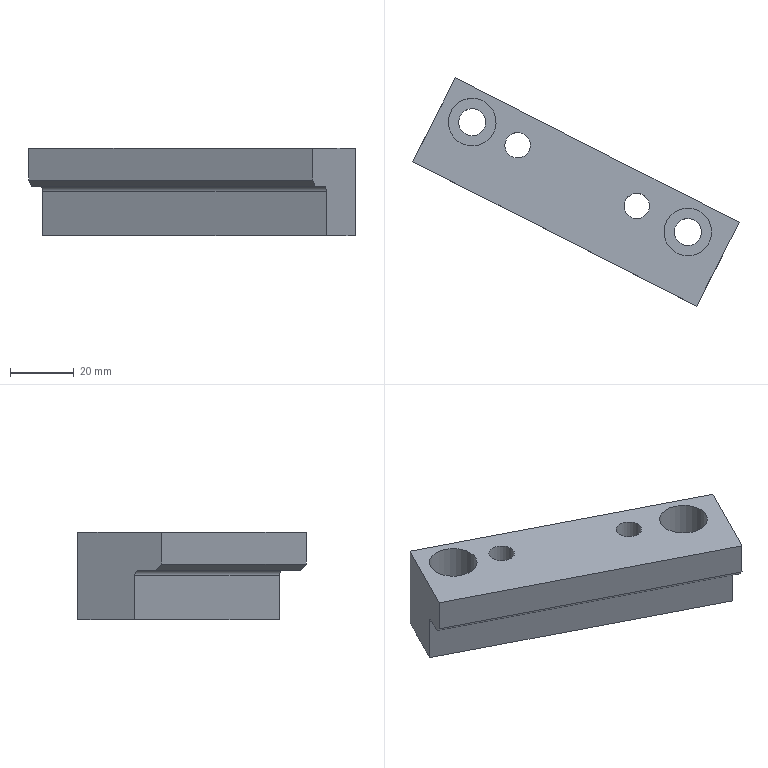Part | STEP file | gslz 2016.10.28-13_id1774_x_t | 1 solid | 18 faces | box 102.493 x 71.684 x 27.5 mm | volume 56764 mm3 | plane 11 | cylinder 7 | commonest cylinder face diameters 8 x2 8.5 x2 15 x2 3 x1
STEP:
#1=CARTESIAN_POINT('',(0.,0.,0.));
#2=DIRECTION('',(0.,0.,1.));
#3=DIRECTION('',(1.,0.,0.));
#4=AXIS2_PLACEMENT_3D('',#1,#2,#3);
#5=CARTESIAN_POINT('',(1106.799,53.815,-63.5));
#6=VERTEX_POINT('',#5);
#7=CARTESIAN_POINT('',(1105.891,52.033,-61.5));
#8=VERTEX_POINT('',#7);
#9=CARTESIAN_POINT('',(1105.891,52.033,-61.5));
#10=DIRECTION('',(-0.321,-0.63,0.7071));
#11=VECTOR('',#10,1.);
#12=LINE('',#9,#11);
#13=CARTESIAN_POINT('',(1154.896,27.063,-61.5));
#14=DIRECTION('',(-0.321,-0.63,-0.7071));
#15=DIRECTION('',(0.2523,-0.7765,0.5774));
#16=AXIS2_PLACEMENT_3D('',#13,#14,#15);
#17=PLANE('',#16);
#18=CARTESIAN_POINT('',(-31.754,44.907));
#19=DIRECTION('',(0.8165,0.5774));
#20=VECTOR('',#19,1.);
#21=LINE('',#18,#20);
#22=(GEOMETRIC_REPRESENTATION_CONTEXT(2)PARAMETRIC_REPRESENTATION_CONTEXT()REPRESENTATION_CONTEXT('',''));
#23=DEFINITIONAL_REPRESENTATION('',(#21),#22);
#24=PCURVE('',#17,#23);
#25=CARTESIAN_POINT('',(1119.283,78.318,-79.639));
#26=DIRECTION('',(0.891,-0.454,0.));
#27=DIRECTION('',(0.454,0.891,0.));
#28=AXIS2_PLACEMENT_3D('',#25,#26,#27);
#29=PLANE('',#28);
#30=CARTESIAN_POINT('',(-29.5,18.139));
#31=DIRECTION('',(-0.7071,0.7071));
#32=VECTOR('',#31,1.);
#33=LINE('',#30,#32);
#34=(GEOMETRIC_REPRESENTATION_CONTEXT(2)PARAMETRIC_REPRESENTATION_CONTEXT()REPRESENTATION_CONTEXT('',''));
#35=DEFINITIONAL_REPRESENTATION('',(#33),#34);
#36=PCURVE('',#29,#35);
#37=SURFACE_CURVE('',#12,(#24,#36),.PCURVE_S1.);
#38=EDGE_CURVE('',#6,#8,#37,.T.);
#39=ORIENTED_EDGE('',*,*,#38,.F.);
#40=CARTESIAN_POINT('',(1195.899,8.416,-63.5));
#41=VERTEX_POINT('',#40);
#42=CARTESIAN_POINT('',(1155.804,28.845,-63.5));
#43=DIRECTION('',(-0.891,0.454,0.));
#44=VECTOR('',#43,1.);
#45=LINE('',#42,#44);
#46=CARTESIAN_POINT('',(-2.309,-1.633));
#47=DIRECTION('',(-0.5774,0.8165));
#48=VECTOR('',#47,1.);
#49=LINE('',#46,#48);
#50=(GEOMETRIC_REPRESENTATION_CONTEXT(2)PARAMETRIC_REPRESENTATION_CONTEXT()REPRESENTATION_CONTEXT('',''));
#51=DEFINITIONAL_REPRESENTATION('',(#49),#50);
#52=PCURVE('',#17,#51);
#53=CARTESIAN_POINT('',(1168.289,53.348,-63.5));
#54=DIRECTION('',(0.,0.,-1.));
#55=DIRECTION('',(0.309,-0.9511,0.));
#56=AXIS2_PLACEMENT_3D('',#53,#54,#55);
#57=PLANE('',#56);
#58=CARTESIAN_POINT('',(19.445,19.445));
#59=DIRECTION('',(-0.7071,0.7071));
#60=VECTOR('',#59,1.);
#61=LINE('',#58,#60);
#62=(GEOMETRIC_REPRESENTATION_CONTEXT(2)PARAMETRIC_REPRESENTATION_CONTEXT()REPRESENTATION_CONTEXT('',''));
#63=DEFINITIONAL_REPRESENTATION('',(#61),#62);
#64=PCURVE('',#57,#63);
#65=SURFACE_CURVE('',#45,(#52,#64),.PCURVE_S1.);
#66=EDGE_CURVE('',#41,#6,#65,.T.);
#67=ORIENTED_EDGE('',*,*,#66,.F.);
#68=CARTESIAN_POINT('',(1194.991,6.634,-61.5));
#69=VERTEX_POINT('',#68);
#70=CARTESIAN_POINT('',(1205.805,27.857,-85.32));
#71=DIRECTION('',(0.321,0.63,-0.7071));
#72=VECTOR('',#71,1.);
#73=LINE('',#70,#72);
#74=CARTESIAN_POINT('',(-1.524,-56.191));
#75=DIRECTION('',(-0.8165,-0.5774));
#76=VECTOR('',#75,1.);
#77=LINE('',#74,#76);
#78=(GEOMETRIC_REPRESENTATION_CONTEXT(2)PARAMETRIC_REPRESENTATION_CONTEXT()REPRESENTATION_CONTEXT('',''));
#79=DEFINITIONAL_REPRESENTATION('',(#77),#78);
#80=PCURVE('',#17,#79);
#81=CARTESIAN_POINT('',(1208.384,32.918,-79.639));
#82=DIRECTION('',(0.891,-0.454,0.));
#83=DIRECTION('',(0.454,0.891,0.));
#84=AXIS2_PLACEMENT_3D('',#81,#82,#83);
#85=PLANE('',#84);
#86=CARTESIAN_POINT('',(-5.68,-5.68));
#87=DIRECTION('',(0.7071,-0.7071));
#88=VECTOR('',#87,1.);
#89=LINE('',#86,#88);
#90=(GEOMETRIC_REPRESENTATION_CONTEXT(2)PARAMETRIC_REPRESENTATION_CONTEXT()REPRESENTATION_CONTEXT('',''));
#91=DEFINITIONAL_REPRESENTATION('',(#89),#90);
#92=PCURVE('',#85,#91);
#93=SURFACE_CURVE('',#73,(#80,#92),.PCURVE_S1.);
#94=EDGE_CURVE('',#69,#41,#93,.T.);
#95=ORIENTED_EDGE('',*,*,#94,.F.);
#96=CARTESIAN_POINT('',(1154.896,27.063,-61.5));
#97=DIRECTION('',(0.891,-0.454,0.));
#98=VECTOR('',#97,1.);
#99=LINE('',#96,#98);
#100=CARTESIAN_POINT('',(0.,0.));
#101=DIRECTION('',(0.5774,-0.8165));
#102=VECTOR('',#101,1.);
#103=LINE('',#100,#102);
#104=(GEOMETRIC_REPRESENTATION_CONTEXT(2)PARAMETRIC_REPRESENTATION_CONTEXT()REPRESENTATION_CONTEXT('',''));
#105=DEFINITIONAL_REPRESENTATION('',(#103),#104);
#106=PCURVE('',#17,#105);
#107=CARTESIAN_POINT('',(1154.896,27.063,-51.5));
#108=DIRECTION('',(0.454,0.891,0.));
#109=DIRECTION('',(-0.891,0.454,0.));
#110=AXIS2_PLACEMENT_3D('',#107,#108,#109);
#111=PLANE('',#110);
#112=CARTESIAN_POINT('',(0.,-10.));
#113=DIRECTION('',(-1.,0.));
#114=VECTOR('',#113,1.);
#115=LINE('',#112,#114);
#116=(GEOMETRIC_REPRESENTATION_CONTEXT(2)PARAMETRIC_REPRESENTATION_CONTEXT()REPRESENTATION_CONTEXT('',''));
#117=DEFINITIONAL_REPRESENTATION('',(#115),#116);
#118=PCURVE('',#111,#117);
#119=SURFACE_CURVE('',#99,(#106,#118),.PCURVE_S1.);
#120=EDGE_CURVE('',#8,#69,#119,.T.);
#121=ORIENTED_EDGE('',*,*,#120,.F.);
#122=EDGE_LOOP('',(#39,#67,#95,#121));
#123=FACE_BOUND('',#122,.T.);
#124=ADVANCED_FACE('',(#123),#17,.T.);
#125=CARTESIAN_POINT('',(1198.623,13.762,-63.5));
#126=VERTEX_POINT('',#125);
#127=CARTESIAN_POINT('',(1208.384,32.918,-63.5));
#128=DIRECTION('',(-0.454,-0.891,0.));
#129=VECTOR('',#128,1.);
#130=LINE('',#127,#129);
#131=CARTESIAN_POINT('',(31.82,-31.82));
#132=DIRECTION('',(0.7071,0.7071));
#133=VECTOR('',#132,1.);
#134=LINE('',#131,#133);
#135=(GEOMETRIC_REPRESENTATION_CONTEXT(2)PARAMETRIC_REPRESENTATION_CONTEXT()REPRESENTATION_CONTEXT('',''));
#136=DEFINITIONAL_REPRESENTATION('',(#134),#135);
#137=PCURVE('',#57,#136);
#138=CARTESIAN_POINT('',(0.,16.139));
#139=DIRECTION('',(-1.,0.));
#140=VECTOR('',#139,1.);
#141=LINE('',#138,#140);
#142=(GEOMETRIC_REPRESENTATION_CONTEXT(2)PARAMETRIC_REPRESENTATION_CONTEXT()REPRESENTATION_CONTEXT('',''));
#143=DEFINITIONAL_REPRESENTATION('',(#141),#142);
#144=PCURVE('',#85,#143);
#145=SURFACE_CURVE('',#130,(#137,#144),.PCURVE_S1.);
#146=EDGE_CURVE('',#126,#41,#145,.T.);
#147=ORIENTED_EDGE('',*,*,#146,.T.);
#148=ORIENTED_EDGE('',*,*,#66,.T.);
#149=CARTESIAN_POINT('',(1109.523,59.161,-63.5));
#150=VERTEX_POINT('',#149);
#151=CARTESIAN_POINT('',(1119.283,78.318,-63.5));
#152=DIRECTION('',(-0.454,-0.891,0.));
#153=VECTOR('',#152,1.);
#154=LINE('',#151,#153);
#155=CARTESIAN_POINT('',(-38.891,38.891));
#156=DIRECTION('',(0.7071,0.7071));
#157=VECTOR('',#156,1.);
#158=LINE('',#155,#157);
#159=(GEOMETRIC_REPRESENTATION_CONTEXT(2)PARAMETRIC_REPRESENTATION_CONTEXT()REPRESENTATION_CONTEXT('',''));
#160=DEFINITIONAL_REPRESENTATION('',(#158),#159);
#161=PCURVE('',#57,#160);
#162=CARTESIAN_POINT('',(0.,16.139));
#163=DIRECTION('',(-1.,0.));
#164=VECTOR('',#163,1.);
#165=LINE('',#162,#164);
#166=(GEOMETRIC_REPRESENTATION_CONTEXT(2)PARAMETRIC_REPRESENTATION_CONTEXT()REPRESENTATION_CONTEXT('',''));
#167=DEFINITIONAL_REPRESENTATION('',(#165),#166);
#168=PCURVE('',#29,#167);
#169=SURFACE_CURVE('',#154,(#161,#168),.PCURVE_S1.);
#170=EDGE_CURVE('',#150,#6,#169,.T.);
#171=ORIENTED_EDGE('',*,*,#170,.F.);
#172=CARTESIAN_POINT('',(1158.528,34.191,-63.5));
#173=DIRECTION('',(0.891,-0.454,0.));
#174=VECTOR('',#173,1.);
#175=LINE('',#172,#174);
#176=CARTESIAN_POINT('',(15.203,15.203));
#177=DIRECTION('',(0.7071,-0.7071));
#178=VECTOR('',#177,1.);
#179=LINE('',#176,#178);
#180=(GEOMETRIC_REPRESENTATION_CONTEXT(2)PARAMETRIC_REPRESENTATION_CONTEXT()REPRESENTATION_CONTEXT('',''));
#181=DEFINITIONAL_REPRESENTATION('',(#179),#180);
#182=PCURVE('',#57,#181);
#183=CARTESIAN_POINT('',(1158.528,34.191,-65.));
#184=DIRECTION('',(0.891,-0.454,0.));
#185=DIRECTION('',(0.454,0.891,0.));
#186=AXIS2_PLACEMENT_3D('',#183,#184,#185);
#187=CYLINDRICAL_SURFACE('',#186,1.5);
#188=CARTESIAN_POINT('',(1.571,0.));
#189=DIRECTION('',(0.,1.));
#190=VECTOR('',#189,1.);
#191=LINE('',#188,#190);
#192=(GEOMETRIC_REPRESENTATION_CONTEXT(2)PARAMETRIC_REPRESENTATION_CONTEXT()REPRESENTATION_CONTEXT('',''));
#193=DEFINITIONAL_REPRESENTATION('',(#191),#192);
#194=PCURVE('',#187,#193);
#195=SURFACE_CURVE('',#175,(#182,#194),.PCURVE_S1.);
#196=EDGE_CURVE('',#150,#126,#195,.T.);
#197=ORIENTED_EDGE('',*,*,#196,.T.);
#198=EDGE_LOOP('',(#147,#148,#171,#197));
#199=FACE_BOUND('',#198,.T.);
#200=ADVANCED_FACE('',(#199),#57,.T.);
#201=ORIENTED_EDGE('',*,*,#196,.T.);
#202=CARTESIAN_POINT('',(1199.304,15.098,-65.));
#203=VERTEX_POINT('',#202);
#204=CARTESIAN_POINT('',(1198.623,13.762,-65.));
#205=DIRECTION('',(-0.891,0.454,0.));
#206=DIRECTION('',(0.454,0.891,0.));
#207=AXIS2_PLACEMENT_3D('',#204,#205,#206);
#208=CIRCLE('',#207,1.5);
#209=CARTESIAN_POINT('',(6.283,45.));
#210=DIRECTION('',(-1.,0.));
#211=VECTOR('',#210,1.);
#212=LINE('',#209,#211);
#213=(GEOMETRIC_REPRESENTATION_CONTEXT(2)PARAMETRIC_REPRESENTATION_CONTEXT()REPRESENTATION_CONTEXT('',''));
#214=DEFINITIONAL_REPRESENTATION('',(#212),#213);
#215=PCURVE('',#187,#214);
#216=CARTESIAN_POINT('',(-20.,14.639));
#217=CARTESIAN_POINT('',(-20.,12.041));
#218=CARTESIAN_POINT('',(-22.25,13.34));
#219=CARTESIAN_POINT('',(-24.5,14.639));
#220=CARTESIAN_POINT('',(-22.25,15.938));
#221=CARTESIAN_POINT('',(-20.,17.237));
#222=CARTESIAN_POINT('',(-20.,14.639));
#223=(BOUNDED_CURVE()B_SPLINE_CURVE(2,(#216,#217,#218,#219,#220,#221,#222),.UNSPECIFIED.,.T.,.F.)B_SPLINE_CURVE_WITH_KNOTS((1,2,2,2,2,1),(-2.094,0.,2.094,4.189,6.283,8.378),.UNSPECIFIED.)CURVE()GEOMETRIC_REPRESENTATION_ITEM()RATIONAL_B_SPLINE_CURVE((1.,0.5,1.,0.5,1.,0.5,1.))REPRESENTATION_ITEM(''));
#224=(GEOMETRIC_REPRESENTATION_CONTEXT(2)PARAMETRIC_REPRESENTATION_CONTEXT()REPRESENTATION_CONTEXT('',''));
#225=DEFINITIONAL_REPRESENTATION('',(#223),#224);
#226=PCURVE('',#85,#225);
#227=SURFACE_CURVE('',#208,(#215,#226),.PCURVE_S1.);
#228=EDGE_CURVE('',#126,#203,#227,.T.);
#229=ORIENTED_EDGE('',*,*,#228,.T.);
#230=CARTESIAN_POINT('',(1110.204,60.497,-65.));
#231=VERTEX_POINT('',#230);
#232=CARTESIAN_POINT('',(1159.209,35.528,-65.));
#233=DIRECTION('',(-0.891,0.454,0.));
#234=VECTOR('',#233,1.);
#235=LINE('',#232,#234);
#236=CARTESIAN_POINT('',(0.,0.));
#237=DIRECTION('',(0.,-1.));
#238=VECTOR('',#237,1.);
#239=LINE('',#236,#238);
#240=(GEOMETRIC_REPRESENTATION_CONTEXT(2)PARAMETRIC_REPRESENTATION_CONTEXT()REPRESENTATION_CONTEXT('',''));
#241=DEFINITIONAL_REPRESENTATION('',(#239),#240);
#242=PCURVE('',#187,#241);
#243=CARTESIAN_POINT('',(1159.209,35.528,-79.639));
#244=DIRECTION('',(0.454,0.891,0.));
#245=DIRECTION('',(-0.891,0.454,0.));
#246=AXIS2_PLACEMENT_3D('',#243,#244,#245);
#247=PLANE('',#246);
#248=CARTESIAN_POINT('',(0.,14.639));
#249=DIRECTION('',(1.,0.));
#250=VECTOR('',#249,1.);
#251=LINE('',#248,#250);
#252=(GEOMETRIC_REPRESENTATION_CONTEXT(2)PARAMETRIC_REPRESENTATION_CONTEXT()REPRESENTATION_CONTEXT('',''));
#253=DEFINITIONAL_REPRESENTATION('',(#251),#252);
#254=PCURVE('',#247,#253);
#255=SURFACE_CURVE('',#235,(#242,#254),.PCURVE_S1.);
#256=EDGE_CURVE('',#203,#231,#255,.T.);
#257=ORIENTED_EDGE('',*,*,#256,.T.);
#258=CARTESIAN_POINT('',(1109.523,59.161,-65.));
#259=DIRECTION('',(0.891,-0.454,0.));
#260=DIRECTION('',(0.454,0.891,0.));
#261=AXIS2_PLACEMENT_3D('',#258,#259,#260);
#262=CIRCLE('',#261,1.5);
#263=CARTESIAN_POINT('',(0.,-55.));
#264=DIRECTION('',(1.,0.));
#265=VECTOR('',#264,1.);
#266=LINE('',#263,#265);
#267=(GEOMETRIC_REPRESENTATION_CONTEXT(2)PARAMETRIC_REPRESENTATION_CONTEXT()REPRESENTATION_CONTEXT('',''));
#268=DEFINITIONAL_REPRESENTATION('',(#266),#267);
#269=PCURVE('',#187,#268);
#270=CARTESIAN_POINT('',(-21.5,14.639));
#271=DIRECTION('',(1.,0.));
#272=AXIS2_PLACEMENT_2D('',#270,#271);
#273=CIRCLE('',#272,1.5);
#274=(GEOMETRIC_REPRESENTATION_CONTEXT(2)PARAMETRIC_REPRESENTATION_CONTEXT()REPRESENTATION_CONTEXT('',''));
#275=DEFINITIONAL_REPRESENTATION('',(#273),#274);
#276=PCURVE('',#29,#275);
#277=SURFACE_CURVE('',#262,(#269,#276),.PCURVE_S1.);
#278=EDGE_CURVE('',#231,#150,#277,.T.);
#279=ORIENTED_EDGE('',*,*,#278,.T.);
#280=EDGE_LOOP('',(#201,#229,#257,#279));
#281=FACE_BOUND('',#280,.F.);
#282=ADVANCED_FACE('',(#281),#187,.F.);
#283=CARTESIAN_POINT('',(1193.574,25.868,-66.5));
#284=VERTEX_POINT('',#283);
#285=CARTESIAN_POINT('',(1192.261,29.91,-66.5));
#286=DIRECTION('',(0.,0.,1.));
#287=DIRECTION('',(0.309,-0.9511,0.));
#288=AXIS2_PLACEMENT_3D('',#285,#286,#287);
#289=CIRCLE('',#288,4.25);
#290=CARTESIAN_POINT('',(1192.261,29.91,-66.5));
#291=DIRECTION('',(0.,0.,-1.));
#292=DIRECTION('',(0.309,-0.9511,0.));
#293=AXIS2_PLACEMENT_3D('',#290,#291,#292);
#294=PLANE('',#293);
#295=CARTESIAN_POINT('',(4.25,0.));
#296=CARTESIAN_POINT('',(4.25,-7.361));
#297=CARTESIAN_POINT('',(-2.125,-3.681));
#298=CARTESIAN_POINT('',(-8.5,0.));
#299=CARTESIAN_POINT('',(-2.125,3.681));
#300=CARTESIAN_POINT('',(4.25,7.361));
#301=CARTESIAN_POINT('',(4.25,0.));
#302=(BOUNDED_CURVE()B_SPLINE_CURVE(2,(#295,#296,#297,#298,#299,#300,#301),.UNSPECIFIED.,.T.,.F.)B_SPLINE_CURVE_WITH_KNOTS((1,2,2,2,2,1),(-2.094,0.,2.094,4.189,6.283,8.378),.UNSPECIFIED.)CURVE()GEOMETRIC_REPRESENTATION_ITEM()RATIONAL_B_SPLINE_CURVE((1.,0.5,1.,0.5,1.,0.5,1.))REPRESENTATION_ITEM(''));
#303=(GEOMETRIC_REPRESENTATION_CONTEXT(2)PARAMETRIC_REPRESENTATION_CONTEXT()REPRESENTATION_CONTEXT('',''));
#304=DEFINITIONAL_REPRESENTATION('',(#302),#303);
#305=PCURVE('',#294,#304);
#306=CARTESIAN_POINT('',(1192.261,29.91,-101.5));
#307=DIRECTION('',(0.,0.,-1.));
#308=DIRECTION('',(0.309,-0.9511,0.));
#309=AXIS2_PLACEMENT_3D('',#306,#307,#308);
#310=CYLINDRICAL_SURFACE('',#309,4.25);
#311=CARTESIAN_POINT('',(6.283,-35.));
#312=DIRECTION('',(-1.,0.));
#313=VECTOR('',#312,1.);
#314=LINE('',#311,#313);
#315=(GEOMETRIC_REPRESENTATION_CONTEXT(2)PARAMETRIC_REPRESENTATION_CONTEXT()REPRESENTATION_CONTEXT('',''));
#316=DEFINITIONAL_REPRESENTATION('',(#314),#315);
#317=PCURVE('',#310,#316);
#318=SURFACE_CURVE('',#289,(#305,#317),.PCURVE_S1.);
#319=EDGE_CURVE('',#284,#284,#318,.T.);
#320=ORIENTED_EDGE('',*,*,#319,.F.);
#321=EDGE_LOOP('',(#320));
#322=FACE_BOUND('',#321,.T.);
#323=CARTESIAN_POINT('',(1194.579,22.777,-66.5));
#324=VERTEX_POINT('',#323);
#325=CARTESIAN_POINT('',(1192.261,29.91,-66.5));
#326=DIRECTION('',(0.,0.,1.));
#327=DIRECTION('',(0.309,-0.9511,0.));
#328=AXIS2_PLACEMENT_3D('',#325,#326,#327);
#329=CIRCLE('',#328,7.5);
#330=CARTESIAN_POINT('',(7.5,0.));
#331=CARTESIAN_POINT('',(7.5,-12.99));
#332=CARTESIAN_POINT('',(-3.75,-6.495));
#333=CARTESIAN_POINT('',(-15.,0.));
#334=CARTESIAN_POINT('',(-3.75,6.495));
#335=CARTESIAN_POINT('',(7.5,12.99));
#336=CARTESIAN_POINT('',(7.5,0.));
#337=(BOUNDED_CURVE()B_SPLINE_CURVE(2,(#330,#331,#332,#333,#334,#335,#336),.UNSPECIFIED.,.T.,.F.)B_SPLINE_CURVE_WITH_KNOTS((1,2,2,2,2,1),(-2.094,0.,2.094,4.189,6.283,8.378),.UNSPECIFIED.)CURVE()GEOMETRIC_REPRESENTATION_ITEM()RATIONAL_B_SPLINE_CURVE((1.,0.5,1.,0.5,1.,0.5,1.))REPRESENTATION_ITEM(''));
#338=(GEOMETRIC_REPRESENTATION_CONTEXT(2)PARAMETRIC_REPRESENTATION_CONTEXT()REPRESENTATION_CONTEXT('',''));
#339=DEFINITIONAL_REPRESENTATION('',(#337),#338);
#340=PCURVE('',#294,#339);
#341=CARTESIAN_POINT('',(1192.261,29.91,-51.5));
#342=DIRECTION('',(0.,0.,-1.));
#343=DIRECTION('',(0.309,-0.9511,0.));
#344=AXIS2_PLACEMENT_3D('',#341,#342,#343);
#345=CYLINDRICAL_SURFACE('',#344,7.5);
#346=CARTESIAN_POINT('',(6.283,15.));
#347=DIRECTION('',(-1.,0.));
#348=VECTOR('',#347,1.);
#349=LINE('',#346,#348);
#350=(GEOMETRIC_REPRESENTATION_CONTEXT(2)PARAMETRIC_REPRESENTATION_CONTEXT()REPRESENTATION_CONTEXT('',''));
#351=DEFINITIONAL_REPRESENTATION('',(#349),#350);
#352=PCURVE('',#345,#351);
#353=SURFACE_CURVE('',#329,(#340,#352),.PCURVE_S1.);
#354=EDGE_CURVE('',#324,#324,#353,.T.);
#355=ORIENTED_EDGE('',*,*,#354,.T.);
#356=EDGE_LOOP('',(#355));
#357=FACE_BOUND('',#356,.T.);
#358=ADVANCED_FACE('',(#322,#357),#294,.F.);
#359=CARTESIAN_POINT('',(1125.858,60.372,-66.5));
#360=VERTEX_POINT('',#359);
#361=CARTESIAN_POINT('',(1124.545,64.414,-66.5));
#362=DIRECTION('',(0.,0.,1.));
#363=DIRECTION('',(0.309,-0.9511,0.));
#364=AXIS2_PLACEMENT_3D('',#361,#362,#363);
#365=CIRCLE('',#364,4.25);
#366=CARTESIAN_POINT('',(1142.365,55.334,-66.5));
#367=DIRECTION('',(0.,0.,-1.));
#368=DIRECTION('',(0.309,-0.9511,0.));
#369=AXIS2_PLACEMENT_3D('',#366,#367,#368);
#370=PLANE('',#369);
#371=CARTESIAN_POINT('',(-9.892,14.142));
#372=CARTESIAN_POINT('',(-9.892,6.781));
#373=CARTESIAN_POINT('',(-16.267,10.462));
#374=CARTESIAN_POINT('',(-22.642,14.142));
#375=CARTESIAN_POINT('',(-16.267,17.823));
#376=CARTESIAN_POINT('',(-9.892,21.503));
#377=CARTESIAN_POINT('',(-9.892,14.142));
#378=(BOUNDED_CURVE()B_SPLINE_CURVE(2,(#371,#372,#373,#374,#375,#376,#377),.UNSPECIFIED.,.T.,.F.)B_SPLINE_CURVE_WITH_KNOTS((1,2,2,2,2,1),(-2.094,0.,2.094,4.189,6.283,8.378),.UNSPECIFIED.)CURVE()GEOMETRIC_REPRESENTATION_ITEM()RATIONAL_B_SPLINE_CURVE((1.,0.5,1.,0.5,1.,0.5,1.))REPRESENTATION_ITEM(''));
#379=(GEOMETRIC_REPRESENTATION_CONTEXT(2)PARAMETRIC_REPRESENTATION_CONTEXT()REPRESENTATION_CONTEXT('',''));
#380=DEFINITIONAL_REPRESENTATION('',(#378),#379);
#381=PCURVE('',#370,#380);
#382=CARTESIAN_POINT('',(1124.545,64.414,-101.5));
#383=DIRECTION('',(0.,0.,-1.));
#384=DIRECTION('',(0.309,-0.9511,0.));
#385=AXIS2_PLACEMENT_3D('',#382,#383,#384);
#386=CYLINDRICAL_SURFACE('',#385,4.25);
#387=CARTESIAN_POINT('',(6.283,-35.));
#388=DIRECTION('',(-1.,0.));
#389=VECTOR('',#388,1.);
#390=LINE('',#387,#389);
#391=(GEOMETRIC_REPRESENTATION_CONTEXT(2)PARAMETRIC_REPRESENTATION_CONTEXT()REPRESENTATION_CONTEXT('',''));
#392=DEFINITIONAL_REPRESENTATION('',(#390),#391);
#393=PCURVE('',#386,#392);
#394=SURFACE_CURVE('',#365,(#381,#393),.PCURVE_S1.);
#395=EDGE_CURVE('',#360,#360,#394,.T.);
#396=ORIENTED_EDGE('',*,*,#395,.F.);
#397=EDGE_LOOP('',(#396));
#398=FACE_BOUND('',#397,.T.);
#399=CARTESIAN_POINT('',(1126.862,57.281,-66.5));
#400=VERTEX_POINT('',#399);
#401=CARTESIAN_POINT('',(1124.545,64.414,-66.5));
#402=DIRECTION('',(0.,0.,1.));
#403=DIRECTION('',(0.309,-0.9511,0.));
#404=AXIS2_PLACEMENT_3D('',#401,#402,#403);
#405=CIRCLE('',#404,7.5);
#406=CARTESIAN_POINT('',(-6.642,14.142));
#407=CARTESIAN_POINT('',(-6.642,1.152));
#408=CARTESIAN_POINT('',(-17.892,7.647));
#409=CARTESIAN_POINT('',(-29.142,14.142));
#410=CARTESIAN_POINT('',(-17.892,20.637));
#411=CARTESIAN_POINT('',(-6.642,27.133));
#412=CARTESIAN_POINT('',(-6.642,14.142));
#413=(BOUNDED_CURVE()B_SPLINE_CURVE(2,(#406,#407,#408,#409,#410,#411,#412),.UNSPECIFIED.,.T.,.F.)B_SPLINE_CURVE_WITH_KNOTS((1,2,2,2,2,1),(-2.094,0.,2.094,4.189,6.283,8.378),.UNSPECIFIED.)CURVE()GEOMETRIC_REPRESENTATION_ITEM()RATIONAL_B_SPLINE_CURVE((1.,0.5,1.,0.5,1.,0.5,1.))REPRESENTATION_ITEM(''));
#414=(GEOMETRIC_REPRESENTATION_CONTEXT(2)PARAMETRIC_REPRESENTATION_CONTEXT()REPRESENTATION_CONTEXT('',''));
#415=DEFINITIONAL_REPRESENTATION('',(#413),#414);
#416=PCURVE('',#370,#415);
#417=CARTESIAN_POINT('',(1124.545,64.414,-51.5));
#418=DIRECTION('',(0.,0.,-1.));
#419=DIRECTION('',(0.309,-0.9511,0.));
#420=AXIS2_PLACEMENT_3D('',#417,#418,#419);
#421=CYLINDRICAL_SURFACE('',#420,7.5);
#422=CARTESIAN_POINT('',(6.283,15.));
#423=DIRECTION('',(-1.,0.));
#424=VECTOR('',#423,1.);
#425=LINE('',#422,#424);
#426=(GEOMETRIC_REPRESENTATION_CONTEXT(2)PARAMETRIC_REPRESENTATION_CONTEXT()REPRESENTATION_CONTEXT('',''));
#427=DEFINITIONAL_REPRESENTATION('',(#425),#426);
#428=PCURVE('',#421,#427);
#429=SURFACE_CURVE('',#405,(#416,#428),.PCURVE_S1.);
#430=EDGE_CURVE('',#400,#400,#429,.T.);
#431=ORIENTED_EDGE('',*,*,#430,.T.);
#432=EDGE_LOOP('',(#431));
#433=FACE_BOUND('',#432,.T.);
#434=ADVANCED_FACE('',(#398,#433),#370,.F.);
#435=CARTESIAN_POINT('',(1194.991,6.634,-51.5));
#436=VERTEX_POINT('',#435);
#437=CARTESIAN_POINT('',(1194.991,6.634,-51.5));
#438=DIRECTION('',(0.,0.,-1.));
#439=VECTOR('',#438,1.);
#440=LINE('',#437,#439);
#441=CARTESIAN_POINT('',(-45.,0.));
#442=DIRECTION('',(0.,-1.));
#443=VECTOR('',#442,1.);
#444=LINE('',#441,#443);
#445=(GEOMETRIC_REPRESENTATION_CONTEXT(2)PARAMETRIC_REPRESENTATION_CONTEXT()REPRESENTATION_CONTEXT('',''));
#446=DEFINITIONAL_REPRESENTATION('',(#444),#445);
#447=PCURVE('',#111,#446);
#448=CARTESIAN_POINT('',(-29.5,28.139));
#449=DIRECTION('',(0.,-1.));
#450=VECTOR('',#449,1.);
#451=LINE('',#448,#450);
#452=(GEOMETRIC_REPRESENTATION_CONTEXT(2)PARAMETRIC_REPRESENTATION_CONTEXT()REPRESENTATION_CONTEXT('',''));
#453=DEFINITIONAL_REPRESENTATION('',(#451),#452);
#454=PCURVE('',#85,#453);
#455=SURFACE_CURVE('',#440,(#447,#454),.PCURVE_S1.);
#456=EDGE_CURVE('',#436,#69,#455,.T.);
#457=ORIENTED_EDGE('',*,*,#456,.F.);
#458=CARTESIAN_POINT('',(1105.891,52.033,-51.5));
#459=VERTEX_POINT('',#458);
#460=CARTESIAN_POINT('',(1154.896,27.063,-51.5));
#461=DIRECTION('',(-0.891,0.454,0.));
#462=VECTOR('',#461,1.);
#463=LINE('',#460,#462);
#464=CARTESIAN_POINT('',(0.,0.));
#465=DIRECTION('',(1.,0.));
#466=VECTOR('',#465,1.);
#467=LINE('',#464,#466);
#468=(GEOMETRIC_REPRESENTATION_CONTEXT(2)PARAMETRIC_REPRESENTATION_CONTEXT()REPRESENTATION_CONTEXT('',''));
#469=DEFINITIONAL_REPRESENTATION('',(#467),#468);
#470=PCURVE('',#111,#469);
#471=CARTESIAN_POINT('',(1168.289,53.348,-51.5));
#472=DIRECTION('',(0.,0.,-1.));
#473=DIRECTION('',(0.309,-0.9511,0.));
#474=AXIS2_PLACEMENT_3D('',#471,#472,#473);
#475=PLANE('',#474);
#476=CARTESIAN_POINT('',(20.86,20.86));
#477=DIRECTION('',(-0.7071,0.7071));
#478=VECTOR('',#477,1.);
#479=LINE('',#476,#478);
#480=(GEOMETRIC_REPRESENTATION_CONTEXT(2)PARAMETRIC_REPRESENTATION_CONTEXT()REPRESENTATION_CONTEXT('',''));
#481=DEFINITIONAL_REPRESENTATION('',(#479),#480);
#482=PCURVE('',#475,#481);
#483=SURFACE_CURVE('',#463,(#470,#482),.PCURVE_S1.);
#484=EDGE_CURVE('',#436,#459,#483,.T.);
#485=ORIENTED_EDGE('',*,*,#484,.T.);
#486=CARTESIAN_POINT('',(1105.891,52.033,-51.5));
#487=DIRECTION('',(0.,0.,-1.));
#488=VECTOR('',#487,1.);
#489=LINE('',#486,#488);
#490=CARTESIAN_POINT('',(55.,0.));
#491=DIRECTION('',(0.,-1.));
#492=VECTOR('',#491,1.);
#493=LINE('',#490,#492);
#494=(GEOMETRIC_REPRESENTATION_CONTEXT(2)PARAMETRIC_REPRESENTATION_CONTEXT()REPRESENTATION_CONTEXT('',''));
#495=DEFINITIONAL_REPRESENTATION('',(#493),#494);
#496=PCURVE('',#111,#495);
#497=CARTESIAN_POINT('',(-29.5,28.139));
#498=DIRECTION('',(0.,-1.));
#499=VECTOR('',#498,1.);
#500=LINE('',#497,#499);
#501=(GEOMETRIC_REPRESENTATION_CONTEXT(2)PARAMETRIC_REPRESENTATION_CONTEXT()REPRESENTATION_CONTEXT('',''));
#502=DEFINITIONAL_REPRESENTATION('',(#500),#501);
#503=PCURVE('',#29,#502);
#504=SURFACE_CURVE('',#489,(#496,#503),.PCURVE_S1.);
#505=EDGE_CURVE('',#459,#8,#504,.T.);
#506=ORIENTED_EDGE('',*,*,#505,.T.);
#507=ORIENTED_EDGE('',*,*,#120,.T.);
#508=EDGE_LOOP('',(#457,#485,#506,#507));
#509=FACE_BOUND('',#508,.T.);
#510=ADVANCED_FACE('',(#509),#111,.F.);
#511=ORIENTED_EDGE('',*,*,#354,.T.);
#512=CARTESIAN_POINT('',(1194.579,22.777,-51.5));
#513=VERTEX_POINT('',#512);
#514=CARTESIAN_POINT('',(1194.579,22.777,-51.5));
#515=CARTESIAN_POINT('',(1194.579,22.777,-66.5));
#516=B_SPLINE_CURVE_WITH_KNOTS('',1,(#514,#515),.UNSPECIFIED.,.F.,.F.,(2,2),(0.,15.),.PIECEWISE_BEZIER_KNOTS.);
#517=CARTESIAN_POINT('',(0.,0.));
#518=DIRECTION('',(0.,1.));
#519=VECTOR('',#518,1.);
#520=LINE('',#517,#519);
#521=(GEOMETRIC_REPRESENTATION_CONTEXT(2)PARAMETRIC_REPRESENTATION_CONTEXT()REPRESENTATION_CONTEXT('',''));
#522=DEFINITIONAL_REPRESENTATION('',(#520),#521);
#523=PCURVE('',#345,#522);
#524=CARTESIAN_POINT('',(6.283,0.));
#525=DIRECTION('',(0.,1.));
#526=VECTOR('',#525,1.);
#527=LINE('',#524,#526);
#528=(GEOMETRIC_REPRESENTATION_CONTEXT(2)PARAMETRIC_REPRESENTATION_CONTEXT()REPRESENTATION_CONTEXT('',''));
#529=DEFINITIONAL_REPRESENTATION('',(#527),#528);
#530=PCURVE('',#345,#529);
#531=SEAM_CURVE('',#516,(#523,#530),.PCURVE_S1.);
#532=EDGE_CURVE('',#513,#324,#531,.T.);
#533=ORIENTED_EDGE('',*,*,#532,.F.);
#534=CARTESIAN_POINT('',(1192.261,29.91,-51.5));
#535=DIRECTION('',(0.,0.,-1.));
#536=DIRECTION('',(0.309,-0.9511,0.));
#537=AXIS2_PLACEMENT_3D('',#534,#535,#536);
#538=CIRCLE('',#537,7.5);
#539=CARTESIAN_POINT('',(0.,0.));
#540=DIRECTION('',(1.,0.));
#541=VECTOR('',#540,1.);
#542=LINE('',#539,#541);
#543=(GEOMETRIC_REPRESENTATION_CONTEXT(2)PARAMETRIC_REPRESENTATION_CONTEXT()REPRESENTATION_CONTEXT('',''));
#544=DEFINITIONAL_REPRESENTATION('',(#542),#543);
#545=PCURVE('',#345,#544);
#546=CARTESIAN_POINT('',(29.698,-15.556));
#547=DIRECTION('',(1.,0.));
#548=AXIS2_PLACEMENT_2D('',#546,#547);
#549=CIRCLE('',#548,7.5);
#550=(GEOMETRIC_REPRESENTATION_CONTEXT(2)PARAMETRIC_REPRESENTATION_CONTEXT()REPRESENTATION_CONTEXT('',''));
#551=DEFINITIONAL_REPRESENTATION('',(#549),#550);
#552=PCURVE('',#475,#551);
#553=SURFACE_CURVE('',#538,(#545,#552),.PCURVE_S1.);
#554=EDGE_CURVE('',#513,#513,#553,.T.);
#555=ORIENTED_EDGE('',*,*,#554,.T.);
#556=ORIENTED_EDGE('',*,*,#532,.T.);
#557=EDGE_LOOP('',(#511,#533,#555,#556));
#558=FACE_BOUND('',#557,.F.);
#559=ADVANCED_FACE('',(#558),#345,.F.);
#560=ORIENTED_EDGE('',*,*,#430,.T.);
#561=CARTESIAN_POINT('',(1126.862,57.281,-51.5));
#562=VERTEX_POINT('',#561);
#563=CARTESIAN_POINT('',(1126.862,57.281,-51.5));
#564=CARTESIAN_POINT('',(1126.862,57.281,-66.5));
#565=B_SPLINE_CURVE_WITH_KNOTS('',1,(#563,#564),.UNSPECIFIED.,.F.,.F.,(2,2),(0.,15.),.PIECEWISE_BEZIER_KNOTS.);
#566=CARTESIAN_POINT('',(0.,0.));
#567=DIRECTION('',(0.,1.));
#568=VECTOR('',#567,1.);
#569=LINE('',#566,#568);
#570=(GEOMETRIC_REPRESENTATION_CONTEXT(2)PARAMETRIC_REPRESENTATION_CONTEXT()REPRESENTATION_CONTEXT('',''));
#571=DEFINITIONAL_REPRESENTATION('',(#569),#570);
#572=PCURVE('',#421,#571);
#573=CARTESIAN_POINT('',(6.283,0.));
#574=DIRECTION('',(0.,1.));
#575=VECTOR('',#574,1.);
#576=LINE('',#573,#575);
#577=(GEOMETRIC_REPRESENTATION_CONTEXT(2)PARAMETRIC_REPRESENTATION_CONTEXT()REPRESENTATION_CONTEXT('',''));
#578=DEFINITIONAL_REPRESENTATION('',(#576),#577);
#579=PCURVE('',#421,#578);
#580=SEAM_CURVE('',#565,(#572,#579),.PCURVE_S1.);
#581=EDGE_CURVE('',#562,#400,#580,.T.);
#582=ORIENTED_EDGE('',*,*,#581,.F.);
#583=CARTESIAN_POINT('',(1124.545,64.414,-51.5));
#584=DIRECTION('',(0.,0.,-1.));
#585=DIRECTION('',(0.309,-0.9511,0.));
#586=AXIS2_PLACEMENT_3D('',#583,#584,#585);
#587=CIRCLE('',#586,7.5);
#588=CARTESIAN_POINT('',(0.,0.));
#589=DIRECTION('',(1.,0.));
#590=VECTOR('',#589,1.);
#591=LINE('',#588,#590);
#592=(GEOMETRIC_REPRESENTATION_CONTEXT(2)PARAMETRIC_REPRESENTATION_CONTEXT()REPRESENTATION_CONTEXT('',''));
#593=DEFINITIONAL_REPRESENTATION('',(#591),#592);
#594=PCURVE('',#421,#593);
#595=CARTESIAN_POINT('',(-24.042,38.184));
#596=DIRECTION('',(1.,0.));
#597=AXIS2_PLACEMENT_2D('',#595,#596);
#598=CIRCLE('',#597,7.5);
#599=(GEOMETRIC_REPRESENTATION_CONTEXT(2)PARAMETRIC_REPRESENTATION_CONTEXT()REPRESENTATION_CONTEXT('',''));
#600=DEFINITIONAL_REPRESENTATION('',(#598),#599);
#601=PCURVE('',#475,#600);
#602=SURFACE_CURVE('',#587,(#594,#601),.PCURVE_S1.);
#603=EDGE_CURVE('',#562,#562,#602,.T.);
#604=ORIENTED_EDGE('',*,*,#603,.T.);
#605=ORIENTED_EDGE('',*,*,#581,.T.);
#606=EDGE_LOOP('',(#560,#582,#604,#605));
#607=FACE_BOUND('',#606,.F.);
#608=ADVANCED_FACE('',(#607),#421,.F.);
#609=CARTESIAN_POINT('',(1208.384,32.918,-51.5));
#610=VERTEX_POINT('',#609);
#611=CARTESIAN_POINT('',(1208.384,32.918,-51.5));
#612=DIRECTION('',(-0.454,-0.891,0.));
#613=VECTOR('',#612,1.);
#614=LINE('',#611,#613);
#615=CARTESIAN_POINT('',(0.,28.139));
#616=DIRECTION('',(-1.,0.));
#617=VECTOR('',#616,1.);
#618=LINE('',#615,#617);
#619=(GEOMETRIC_REPRESENTATION_CONTEXT(2)PARAMETRIC_REPRESENTATION_CONTEXT()REPRESENTATION_CONTEXT('',''));
#620=DEFINITIONAL_REPRESENTATION('',(#618),#619);
#621=PCURVE('',#85,#620);
#622=CARTESIAN_POINT('',(31.82,-31.82));
#623=DIRECTION('',(0.7071,0.7071));
#624=VECTOR('',#623,1.);
#625=LINE('',#622,#624);
#626=(GEOMETRIC_REPRESENTATION_CONTEXT(2)PARAMETRIC_REPRESENTATION_CONTEXT()REPRESENTATION_CONTEXT('',''));
#627=DEFINITIONAL_REPRESENTATION('',(#625),#626);
#628=PCURVE('',#475,#627);
#629=SURFACE_CURVE('',#614,(#621,#628),.PCURVE_S1.);
#630=EDGE_CURVE('',#610,#436,#629,.T.);
#631=ORIENTED_EDGE('',*,*,#630,.T.);
#632=ORIENTED_EDGE('',*,*,#456,.T.);
#633=ORIENTED_EDGE('',*,*,#94,.T.);
#634=ORIENTED_EDGE('',*,*,#146,.F.);
#635=ORIENTED_EDGE('',*,*,#228,.T.);
#636=CARTESIAN_POINT('',(1199.304,15.098,-79.));
#637=VERTEX_POINT('',#636);
#638=CARTESIAN_POINT('',(1199.304,15.098,-79.639));
#639=DIRECTION('',(0.,0.,1.));
#640=VECTOR('',#639,1.);
#641=LINE('',#638,#640);
#642=CARTESIAN_POINT('',(-20.,0.));
#643=DIRECTION('',(0.,1.));
#644=VECTOR('',#643,1.);
#645=LINE('',#642,#644);
#646=(GEOMETRIC_REPRESENTATION_CONTEXT(2)PARAMETRIC_REPRESENTATION_CONTEXT()REPRESENTATION_CONTEXT('',''));
#647=DEFINITIONAL_REPRESENTATION('',(#645),#646);
#648=PCURVE('',#85,#647);
#649=CARTESIAN_POINT('',(-45.,0.));
#650=DIRECTION('',(0.,1.));
#651=VECTOR('',#650,1.);
#652=LINE('',#649,#651);
#653=(GEOMETRIC_REPRESENTATION_CONTEXT(2)PARAMETRIC_REPRESENTATION_CONTEXT()REPRESENTATION_CONTEXT('',''));
#654=DEFINITIONAL_REPRESENTATION('',(#652),#653);
#655=PCURVE('',#247,#654);
#656=SURFACE_CURVE('',#641,(#648,#655),.PCURVE_S1.);
#657=EDGE_CURVE('',#637,#203,#656,.T.);
#658=ORIENTED_EDGE('',*,*,#657,.F.);
#659=CARTESIAN_POINT('',(1208.384,32.918,-79.));
#660=VERTEX_POINT('',#659);
#661=CARTESIAN_POINT('',(1208.384,32.918,-79.));
#662=DIRECTION('',(-0.454,-0.891,0.));
#663=VECTOR('',#662,1.);
#664=LINE('',#661,#663);
#665=CARTESIAN_POINT('',(0.,0.6394));
#666=DIRECTION('',(-1.,0.));
#667=VECTOR('',#666,1.);
#668=LINE('',#665,#667);
#669=(GEOMETRIC_REPRESENTATION_CONTEXT(2)PARAMETRIC_REPRESENTATION_CONTEXT()REPRESENTATION_CONTEXT('',''));
#670=DEFINITIONAL_REPRESENTATION('',(#668),#669);
#671=PCURVE('',#85,#670);
#672=CARTESIAN_POINT('',(1168.289,53.348,-79.));
#673=DIRECTION('',(0.,0.,-1.));
#674=DIRECTION('',(0.309,-0.9511,0.));
#675=AXIS2_PLACEMENT_3D('',#672,#673,#674);
#676=PLANE('',#675);
#677=CARTESIAN_POINT('',(31.82,-31.82));
#678=DIRECTION('',(0.7071,0.7071));
#679=VECTOR('',#678,1.);
#680=LINE('',#677,#679);
#681=(GEOMETRIC_REPRESENTATION_CONTEXT(2)PARAMETRIC_REPRESENTATION_CONTEXT()REPRESENTATION_CONTEXT('',''));
#682=DEFINITIONAL_REPRESENTATION('',(#680),#681);
#683=PCURVE('',#676,#682);
#684=SURFACE_CURVE('',#664,(#671,#683),.PCURVE_S1.);
#685=EDGE_CURVE('',#660,#637,#684,.T.);
#686=ORIENTED_EDGE('',*,*,#685,.F.);
#687=CARTESIAN_POINT('',(1208.384,32.918,-79.639));
#688=DIRECTION('',(0.,0.,1.));
#689=VECTOR('',#688,1.);
#690=LINE('',#687,#689);
#691=CARTESIAN_POINT('',(0.,0.));
#692=DIRECTION('',(0.,1.));
#693=VECTOR('',#692,1.);
#694=LINE('',#691,#693);
#695=(GEOMETRIC_REPRESENTATION_CONTEXT(2)PARAMETRIC_REPRESENTATION_CONTEXT()REPRESENTATION_CONTEXT('',''));
#696=DEFINITIONAL_REPRESENTATION('',(#694),#695);
#697=PCURVE('',#85,#696);
#698=CARTESIAN_POINT('',(1168.289,53.348,-79.639));
#699=DIRECTION('',(0.454,0.891,0.));
#700=DIRECTION('',(-0.891,0.454,0.));
#701=AXIS2_PLACEMENT_3D('',#698,#699,#700);
#702=PLANE('',#701);
#703=CARTESIAN_POINT('',(-45.,0.));
#704=DIRECTION('',(0.,1.));
#705=VECTOR('',#704,1.);
#706=LINE('',#703,#705);
#707=(GEOMETRIC_REPRESENTATION_CONTEXT(2)PARAMETRIC_REPRESENTATION_CONTEXT()REPRESENTATION_CONTEXT('',''));
#708=DEFINITIONAL_REPRESENTATION('',(#706),#707);
#709=PCURVE('',#702,#708);
#710=SURFACE_CURVE('',#690,(#697,#709),.PCURVE_S1.);
#711=EDGE_CURVE('',#660,#610,#710,.T.);
#712=ORIENTED_EDGE('',*,*,#711,.T.);
#713=EDGE_LOOP('',(#631,#632,#633,#634,#635,#658,#686,#712));
#714=FACE_BOUND('',#713,.T.);
#715=ADVANCED_FACE('',(#714),#85,.T.);
#716=CARTESIAN_POINT('',(1119.283,78.318,-79.));
#717=VERTEX_POINT('',#716);
#718=CARTESIAN_POINT('',(1119.283,78.318,-51.5));
#719=VERTEX_POINT('',#718);
#720=CARTESIAN_POINT('',(1119.283,78.318,-79.639));
#721=DIRECTION('',(0.,0.,1.));
#722=VECTOR('',#721,1.);
#723=LINE('',#720,#722);
#724=CARTESIAN_POINT('',(55.,0.));
#725=DIRECTION('',(0.,1.));
#726=VECTOR('',#725,1.);
#727=LINE('',#724,#726);
#728=(GEOMETRIC_REPRESENTATION_CONTEXT(2)PARAMETRIC_REPRESENTATION_CONTEXT()REPRESENTATION_CONTEXT('',''));
#729=DEFINITIONAL_REPRESENTATION('',(#727),#728);
#730=PCURVE('',#702,#729);
#731=CARTESIAN_POINT('',(0.,0.));
#732=DIRECTION('',(0.,1.));
#733=VECTOR('',#732,1.);
#734=LINE('',#731,#733);
#735=(GEOMETRIC_REPRESENTATION_CONTEXT(2)PARAMETRIC_REPRESENTATION_CONTEXT()REPRESENTATION_CONTEXT('',''));
#736=DEFINITIONAL_REPRESENTATION('',(#734),#735);
#737=PCURVE('',#29,#736);
#738=SURFACE_CURVE('',#723,(#730,#737),.PCURVE_S1.);
#739=EDGE_CURVE('',#717,#719,#738,.T.);
#740=ORIENTED_EDGE('',*,*,#739,.T.);
#741=CARTESIAN_POINT('',(1168.289,53.348,-51.5));
#742=DIRECTION('',(-0.891,0.454,0.));
#743=VECTOR('',#742,1.);
#744=LINE('',#741,#743);
#745=CARTESIAN_POINT('',(0.,28.139));
#746=DIRECTION('',(1.,0.));
#747=VECTOR('',#746,1.);
#748=LINE('',#745,#747);
#749=(GEOMETRIC_REPRESENTATION_CONTEXT(2)PARAMETRIC_REPRESENTATION_CONTEXT()REPRESENTATION_CONTEXT('',''));
#750=DEFINITIONAL_REPRESENTATION('',(#748),#749);
#751=PCURVE('',#702,#750);
#752=CARTESIAN_POINT('',(0.,0.));
#753=DIRECTION('',(-0.7071,0.7071));
#754=VECTOR('',#753,1.);
#755=LINE('',#752,#754);
#756=(GEOMETRIC_REPRESENTATION_CONTEXT(2)PARAMETRIC_REPRESENTATION_CONTEXT()REPRESENTATION_CONTEXT('',''));
#757=DEFINITIONAL_REPRESENTATION('',(#755),#756);
#758=PCURVE('',#475,#757);
#759=SURFACE_CURVE('',#744,(#751,#758),.PCURVE_S1.);
#760=EDGE_CURVE('',#610,#719,#759,.T.);
#761=ORIENTED_EDGE('',*,*,#760,.F.);
#762=ORIENTED_EDGE('',*,*,#711,.F.);
#763=CARTESIAN_POINT('',(1168.289,53.348,-79.));
#764=DIRECTION('',(0.891,-0.454,0.));
#765=VECTOR('',#764,1.);
#766=LINE('',#763,#765);
#767=CARTESIAN_POINT('',(0.,0.6394));
#768=DIRECTION('',(-1.,0.));
#769=VECTOR('',#768,1.);
#770=LINE('',#767,#769);
#771=(GEOMETRIC_REPRESENTATION_CONTEXT(2)PARAMETRIC_REPRESENTATION_CONTEXT()REPRESENTATION_CONTEXT('',''));
#772=DEFINITIONAL_REPRESENTATION('',(#770),#771);
#773=PCURVE('',#702,#772);
#774=CARTESIAN_POINT('',(0.,0.));
#775=DIRECTION('',(0.7071,-0.7071));
#776=VECTOR('',#775,1.);
#777=LINE('',#774,#776);
#778=(GEOMETRIC_REPRESENTATION_CONTEXT(2)PARAMETRIC_REPRESENTATION_CONTEXT()REPRESENTATION_CONTEXT('',''));
#779=DEFINITIONAL_REPRESENTATION('',(#777),#778);
#780=PCURVE('',#676,#779);
#781=SURFACE_CURVE('',#766,(#773,#780),.PCURVE_S1.);
#782=EDGE_CURVE('',#717,#660,#781,.T.);
#783=ORIENTED_EDGE('',*,*,#782,.F.);
#784=EDGE_LOOP('',(#740,#761,#762,#783));
#785=FACE_BOUND('',#784,.T.);
#786=ADVANCED_FACE('',(#785),#702,.T.);
#787=ORIENTED_EDGE('',*,*,#505,.F.);
#788=CARTESIAN_POINT('',(1119.283,78.318,-51.5));
#789=DIRECTION('',(-0.454,-0.891,0.));
#790=VECTOR('',#789,1.);
#791=LINE('',#788,#790);
#792=CARTESIAN_POINT('',(0.,28.139));
#793=DIRECTION('',(-1.,0.));
#794=VECTOR('',#793,1.);
#795=LINE('',#792,#794);
#796=(GEOMETRIC_REPRESENTATION_CONTEXT(2)PARAMETRIC_REPRESENTATION_CONTEXT()REPRESENTATION_CONTEXT('',''));
#797=DEFINITIONAL_REPRESENTATION('',(#795),#796);
#798=PCURVE('',#29,#797);
#799=CARTESIAN_POINT('',(-38.891,38.891));
#800=DIRECTION('',(0.7071,0.7071));
#801=VECTOR('',#800,1.);
#802=LINE('',#799,#801);
#803=(GEOMETRIC_REPRESENTATION_CONTEXT(2)PARAMETRIC_REPRESENTATION_CONTEXT()REPRESENTATION_CONTEXT('',''));
#804=DEFINITIONAL_REPRESENTATION('',(#802),#803);
#805=PCURVE('',#475,#804);
#806=SURFACE_CURVE('',#791,(#798,#805),.PCURVE_S1.);
#807=EDGE_CURVE('',#719,#459,#806,.T.);
#808=ORIENTED_EDGE('',*,*,#807,.F.);
#809=ORIENTED_EDGE('',*,*,#739,.F.);
#810=CARTESIAN_POINT('',(1110.204,60.497,-79.));
#811=VERTEX_POINT('',#810);
#812=CARTESIAN_POINT('',(1119.283,78.318,-79.));
#813=DIRECTION('',(-0.454,-0.891,0.));
#814=VECTOR('',#813,1.);
#815=LINE('',#812,#814);
#816=CARTESIAN_POINT('',(0.,0.6394));
#817=DIRECTION('',(-1.,0.));
#818=VECTOR('',#817,1.);
#819=LINE('',#816,#818);
#820=(GEOMETRIC_REPRESENTATION_CONTEXT(2)PARAMETRIC_REPRESENTATION_CONTEXT()REPRESENTATION_CONTEXT('',''));
#821=DEFINITIONAL_REPRESENTATION('',(#819),#820);
#822=PCURVE('',#29,#821);
#823=CARTESIAN_POINT('',(-38.891,38.891));
#824=DIRECTION('',(0.7071,0.7071));
#825=VECTOR('',#824,1.);
#826=LINE('',#823,#825);
#827=(GEOMETRIC_REPRESENTATION_CONTEXT(2)PARAMETRIC_REPRESENTATION_CONTEXT()REPRESENTATION_CONTEXT('',''));
#828=DEFINITIONAL_REPRESENTATION('',(#826),#827);
#829=PCURVE('',#676,#828);
#830=SURFACE_CURVE('',#815,(#822,#829),.PCURVE_S1.);
#831=EDGE_CURVE('',#717,#811,#830,.T.);
#832=ORIENTED_EDGE('',*,*,#831,.T.);
#833=CARTESIAN_POINT('',(1110.204,60.497,-79.639));
#834=DIRECTION('',(0.,0.,1.));
#835=VECTOR('',#834,1.);
#836=LINE('',#833,#835);
#837=CARTESIAN_POINT('',(-20.,0.));
#838=DIRECTION('',(0.,1.));
#839=VECTOR('',#838,1.);
#840=LINE('',#837,#839);
#841=(GEOMETRIC_REPRESENTATION_CONTEXT(2)PARAMETRIC_REPRESENTATION_CONTEXT()REPRESENTATION_CONTEXT('',''));
#842=DEFINITIONAL_REPRESENTATION('',(#840),#841);
#843=PCURVE('',#29,#842);
#844=CARTESIAN_POINT('',(55.,0.));
#845=DIRECTION('',(0.,1.));
#846=VECTOR('',#845,1.);
#847=LINE('',#844,#846);
#848=(GEOMETRIC_REPRESENTATION_CONTEXT(2)PARAMETRIC_REPRESENTATION_CONTEXT()REPRESENTATION_CONTEXT('',''));
#849=DEFINITIONAL_REPRESENTATION('',(#847),#848);
#850=PCURVE('',#247,#849);
#851=SURFACE_CURVE('',#836,(#843,#850),.PCURVE_S1.);
#852=EDGE_CURVE('',#811,#231,#851,.T.);
#853=ORIENTED_EDGE('',*,*,#852,.T.);
#854=ORIENTED_EDGE('',*,*,#278,.T.);
#855=ORIENTED_EDGE('',*,*,#170,.T.);
#856=ORIENTED_EDGE('',*,*,#38,.T.);
#857=EDGE_LOOP('',(#787,#808,#809,#832,#853,#854,#855,#856));
#858=FACE_BOUND('',#857,.T.);
#859=ADVANCED_FACE('',(#858),#29,.F.);
#860=ORIENTED_EDGE('',*,*,#657,.T.);
#861=ORIENTED_EDGE('',*,*,#256,.T.);
#862=ORIENTED_EDGE('',*,*,#852,.F.);
#863=CARTESIAN_POINT('',(1159.209,35.528,-79.));
#864=DIRECTION('',(0.891,-0.454,0.));
#865=VECTOR('',#864,1.);
#866=LINE('',#863,#865);
#867=CARTESIAN_POINT('',(0.,0.6394));
#868=DIRECTION('',(-1.,0.));
#869=VECTOR('',#868,1.);
#870=LINE('',#867,#869);
#871=(GEOMETRIC_REPRESENTATION_CONTEXT(2)PARAMETRIC_REPRESENTATION_CONTEXT()REPRESENTATION_CONTEXT('',''));
#872=DEFINITIONAL_REPRESENTATION('',(#870),#871);
#873=PCURVE('',#247,#872);
#874=CARTESIAN_POINT('',(14.142,14.142));
#875=DIRECTION('',(0.7071,-0.7071));
#876=VECTOR('',#875,1.);
#877=LINE('',#874,#876);
#878=(GEOMETRIC_REPRESENTATION_CONTEXT(2)PARAMETRIC_REPRESENTATION_CONTEXT()REPRESENTATION_CONTEXT('',''));
#879=DEFINITIONAL_REPRESENTATION('',(#877),#878);
#880=PCURVE('',#676,#879);
#881=SURFACE_CURVE('',#866,(#873,#880),.PCURVE_S1.);
#882=EDGE_CURVE('',#811,#637,#881,.T.);
#883=ORIENTED_EDGE('',*,*,#882,.T.);
#884=EDGE_LOOP('',(#860,#861,#862,#883));
#885=FACE_BOUND('',#884,.T.);
#886=ADVANCED_FACE('',(#885),#247,.F.);
#887=CARTESIAN_POINT('',(1193.574,25.868,-79.));
#888=VERTEX_POINT('',#887);
#889=CARTESIAN_POINT('',(1192.261,29.91,-79.));
#890=DIRECTION('',(0.,0.,-1.));
#891=DIRECTION('',(0.309,-0.9511,0.));
#892=AXIS2_PLACEMENT_3D('',#889,#890,#891);
#893=CIRCLE('',#892,4.25);
#894=CARTESIAN_POINT('',(0.,-22.5));
#895=DIRECTION('',(1.,0.));
#896=VECTOR('',#895,1.);
#897=LINE('',#894,#896);
#898=(GEOMETRIC_REPRESENTATION_CONTEXT(2)PARAMETRIC_REPRESENTATION_CONTEXT()REPRESENTATION_CONTEXT('',''));
#899=DEFINITIONAL_REPRESENTATION('',(#897),#898);
#900=PCURVE('',#310,#899);
#901=CARTESIAN_POINT('',(29.698,-15.556));
#902=DIRECTION('',(1.,0.));
#903=AXIS2_PLACEMENT_2D('',#901,#902);
#904=CIRCLE('',#903,4.25);
#905=(GEOMETRIC_REPRESENTATION_CONTEXT(2)PARAMETRIC_REPRESENTATION_CONTEXT()REPRESENTATION_CONTEXT('',''));
#906=DEFINITIONAL_REPRESENTATION('',(#904),#905);
#907=PCURVE('',#676,#906);
#908=SURFACE_CURVE('',#893,(#900,#907),.PCURVE_S1.);
#909=EDGE_CURVE('',#888,#888,#908,.T.);
#910=ORIENTED_EDGE('',*,*,#909,.F.);
#911=CARTESIAN_POINT('',(1193.574,25.868,-66.5));
#912=CARTESIAN_POINT('',(1193.574,25.868,-79.));
#913=B_SPLINE_CURVE_WITH_KNOTS('',1,(#911,#912),.UNSPECIFIED.,.F.,.F.,(2,2),(-35.,-22.5),.PIECEWISE_BEZIER_KNOTS.);
#914=CARTESIAN_POINT('',(0.,0.));
#915=DIRECTION('',(0.,1.));
#916=VECTOR('',#915,1.);
#917=LINE('',#914,#916);
#918=(GEOMETRIC_REPRESENTATION_CONTEXT(2)PARAMETRIC_REPRESENTATION_CONTEXT()REPRESENTATION_CONTEXT('',''));
#919=DEFINITIONAL_REPRESENTATION('',(#917),#918);
#920=PCURVE('',#310,#919);
#921=CARTESIAN_POINT('',(6.283,0.));
#922=DIRECTION('',(0.,1.));
#923=VECTOR('',#922,1.);
#924=LINE('',#921,#923);
#925=(GEOMETRIC_REPRESENTATION_CONTEXT(2)PARAMETRIC_REPRESENTATION_CONTEXT()REPRESENTATION_CONTEXT('',''));
#926=DEFINITIONAL_REPRESENTATION('',(#924),#925);
#927=PCURVE('',#310,#926);
#928=SEAM_CURVE('',#913,(#920,#927),.PCURVE_S1.);
#929=EDGE_CURVE('',#284,#888,#928,.T.);
#930=ORIENTED_EDGE('',*,*,#929,.F.);
#931=ORIENTED_EDGE('',*,*,#319,.F.);
#932=ORIENTED_EDGE('',*,*,#929,.T.);
#933=EDGE_LOOP('',(#910,#930,#931,#932));
#934=FACE_BOUND('',#933,.F.);
#935=ADVANCED_FACE('',(#934),#310,.F.);
#936=CARTESIAN_POINT('',(1125.858,60.372,-79.));
#937=VERTEX_POINT('',#936);
#938=CARTESIAN_POINT('',(1124.545,64.414,-79.));
#939=DIRECTION('',(0.,0.,-1.));
#940=DIRECTION('',(0.309,-0.9511,0.));
#941=AXIS2_PLACEMENT_3D('',#938,#939,#940);
#942=CIRCLE('',#941,4.25);
#943=CARTESIAN_POINT('',(0.,-22.5));
#944=DIRECTION('',(1.,0.));
#945=VECTOR('',#944,1.);
#946=LINE('',#943,#945);
#947=(GEOMETRIC_REPRESENTATION_CONTEXT(2)PARAMETRIC_REPRESENTATION_CONTEXT()REPRESENTATION_CONTEXT('',''));
#948=DEFINITIONAL_REPRESENTATION('',(#946),#947);
#949=PCURVE('',#386,#948);
#950=CARTESIAN_POINT('',(-24.042,38.184));
#951=DIRECTION('',(1.,0.));
#952=AXIS2_PLACEMENT_2D('',#950,#951);
#953=CIRCLE('',#952,4.25);
#954=(GEOMETRIC_REPRESENTATION_CONTEXT(2)PARAMETRIC_REPRESENTATION_CONTEXT()REPRESENTATION_CONTEXT('',''));
#955=DEFINITIONAL_REPRESENTATION('',(#953),#954);
#956=PCURVE('',#676,#955);
#957=SURFACE_CURVE('',#942,(#949,#956),.PCURVE_S1.);
#958=EDGE_CURVE('',#937,#937,#957,.T.);
#959=ORIENTED_EDGE('',*,*,#958,.F.);
#960=CARTESIAN_POINT('',(1125.858,60.372,-66.5));
#961=CARTESIAN_POINT('',(1125.858,60.372,-79.));
#962=B_SPLINE_CURVE_WITH_KNOTS('',1,(#960,#961),.UNSPECIFIED.,.F.,.F.,(2,2),(-35.,-22.5),.PIECEWISE_BEZIER_KNOTS.);
#963=CARTESIAN_POINT('',(0.,0.));
#964=DIRECTION('',(0.,1.));
#965=VECTOR('',#964,1.);
#966=LINE('',#963,#965);
#967=(GEOMETRIC_REPRESENTATION_CONTEXT(2)PARAMETRIC_REPRESENTATION_CONTEXT()REPRESENTATION_CONTEXT('',''));
#968=DEFINITIONAL_REPRESENTATION('',(#966),#967);
#969=PCURVE('',#386,#968);
#970=CARTESIAN_POINT('',(6.283,0.));
#971=DIRECTION('',(0.,1.));
#972=VECTOR('',#971,1.);
#973=LINE('',#970,#972);
#974=(GEOMETRIC_REPRESENTATION_CONTEXT(2)PARAMETRIC_REPRESENTATION_CONTEXT()REPRESENTATION_CONTEXT('',''));
#975=DEFINITIONAL_REPRESENTATION('',(#973),#974);
#976=PCURVE('',#386,#975);
#977=SEAM_CURVE('',#962,(#969,#976),.PCURVE_S1.);
#978=EDGE_CURVE('',#360,#937,#977,.T.);
#979=ORIENTED_EDGE('',*,*,#978,.F.);
#980=ORIENTED_EDGE('',*,*,#395,.F.);
#981=ORIENTED_EDGE('',*,*,#978,.T.);
#982=EDGE_LOOP('',(#959,#979,#980,#981));
#983=FACE_BOUND('',#982,.F.);
#984=ADVANCED_FACE('',(#983),#386,.F.);
#985=CARTESIAN_POINT('',(1135.649,54.687,-51.5));
#986=VERTEX_POINT('',#985);
#987=CARTESIAN_POINT('',(1138.801,57.15,-51.5));
#988=DIRECTION('',(0.,0.,-1.));
#989=DIRECTION('',(-0.788,-0.6157,0.));
#990=AXIS2_PLACEMENT_3D('',#987,#988,#989);
#991=CIRCLE('',#990,4.);
#992=CARTESIAN_POINT('',(1138.801,57.15,-101.5));
#993=DIRECTION('',(0.,0.,-1.));
#994=DIRECTION('',(0.309,-0.9511,0.));
#995=AXIS2_PLACEMENT_3D('',#992,#993,#994);
#996=CYLINDRICAL_SURFACE('',#995,4.);
#997=CARTESIAN_POINT('',(1.222,-50.));
#998=DIRECTION('',(1.,0.));
#999=VECTOR('',#998,1.);
#1000=LINE('',#997,#999);
#1001=(GEOMETRIC_REPRESENTATION_CONTEXT(2)PARAMETRIC_REPRESENTATION_CONTEXT()REPRESENTATION_CONTEXT('',''));
#1002=DEFINITIONAL_REPRESENTATION('',(#1000),#1001);
#1003=PCURVE('',#996,#1002);
#1004=CARTESIAN_POINT('',(-12.728,26.87));
#1005=DIRECTION('',(0.342,0.9397));
#1006=AXIS2_PLACEMENT_2D('',#1004,#1005);
#1007=CIRCLE('',#1006,4.);
#1008=(GEOMETRIC_REPRESENTATION_CONTEXT(2)PARAMETRIC_REPRESENTATION_CONTEXT()REPRESENTATION_CONTEXT('',''));
#1009=DEFINITIONAL_REPRESENTATION('',(#1007),#1008);
#1010=PCURVE('',#475,#1009);
#1011=SURFACE_CURVE('',#991,(#1003,#1010),.PCURVE_S1.);
#1012=EDGE_CURVE('',#986,#986,#1011,.T.);
#1013=ORIENTED_EDGE('',*,*,#1012,.T.);
#1014=CARTESIAN_POINT('',(1135.649,54.687,-79.));
#1015=VERTEX_POINT('',#1014);
#1016=CARTESIAN_POINT('',(1135.649,54.687,-51.5));
#1017=CARTESIAN_POINT('',(1135.649,54.687,-79.));
#1018=B_SPLINE_CURVE_WITH_KNOTS('',1,(#1016,#1017),.UNSPECIFIED.,.F.,.F.,(2,2),(-50.,-22.5),.PIECEWISE_BEZIER_KNOTS.);
#1019=CARTESIAN_POINT('',(7.505,0.));
#1020=DIRECTION('',(0.,1.));
#1021=VECTOR('',#1020,1.);
#1022=LINE('',#1019,#1021);
#1023=(GEOMETRIC_REPRESENTATION_CONTEXT(2)PARAMETRIC_REPRESENTATION_CONTEXT()REPRESENTATION_CONTEXT('',''));
#1024=DEFINITIONAL_REPRESENTATION('',(#1022),#1023);
#1025=PCURVE('',#996,#1024);
#1026=CARTESIAN_POINT('',(1.222,0.));
#1027=DIRECTION('',(0.,1.));
#1028=VECTOR('',#1027,1.);
#1029=LINE('',#1026,#1028);
#1030=(GEOMETRIC_REPRESENTATION_CONTEXT(2)PARAMETRIC_REPRESENTATION_CONTEXT()REPRESENTATION_CONTEXT('',''));
#1031=DEFINITIONAL_REPRESENTATION('',(#1029),#1030);
#1032=PCURVE('',#996,#1031);
#1033=SEAM_CURVE('',#1018,(#1025,#1032),.PCURVE_S1.);
#1034=EDGE_CURVE('',#986,#1015,#1033,.T.);
#1035=ORIENTED_EDGE('',*,*,#1034,.T.);
#1036=CARTESIAN_POINT('',(1138.801,57.15,-79.));
#1037=DIRECTION('',(0.,0.,-1.));
#1038=DIRECTION('',(-0.788,-0.6157,0.));
#1039=AXIS2_PLACEMENT_3D('',#1036,#1037,#1038);
#1040=CIRCLE('',#1039,4.);
#1041=CARTESIAN_POINT('',(1.222,-22.5));
#1042=DIRECTION('',(1.,0.));
#1043=VECTOR('',#1042,1.);
#1044=LINE('',#1041,#1043);
#1045=(GEOMETRIC_REPRESENTATION_CONTEXT(2)PARAMETRIC_REPRESENTATION_CONTEXT()REPRESENTATION_CONTEXT('',''));
#1046=DEFINITIONAL_REPRESENTATION('',(#1044),#1045);
#1047=PCURVE('',#996,#1046);
#1048=CARTESIAN_POINT('',(-12.728,26.87));
#1049=DIRECTION('',(0.342,0.9397));
#1050=AXIS2_PLACEMENT_2D('',#1048,#1049);
#1051=CIRCLE('',#1050,4.);
#1052=(GEOMETRIC_REPRESENTATION_CONTEXT(2)PARAMETRIC_REPRESENTATION_CONTEXT()REPRESENTATION_CONTEXT('',''));
#1053=DEFINITIONAL_REPRESENTATION('',(#1051),#1052);
#1054=PCURVE('',#676,#1053);
#1055=SURFACE_CURVE('',#1040,(#1047,#1054),.PCURVE_S1.);
#1056=EDGE_CURVE('',#1015,#1015,#1055,.T.);
#1057=ORIENTED_EDGE('',*,*,#1056,.F.);
#1058=ORIENTED_EDGE('',*,*,#1034,.F.);
#1059=EDGE_LOOP('',(#1013,#1035,#1057,#1058));
#1060=FACE_BOUND('',#1059,.F.);
#1061=ADVANCED_FACE('',(#1060),#996,.F.);
#1062=CARTESIAN_POINT('',(1173.071,35.619,-79.));
#1063=VERTEX_POINT('',#1062);
#1064=CARTESIAN_POINT('',(1176.223,38.082,-79.));
#1065=DIRECTION('',(0.,0.,-1.));
#1066=DIRECTION('',(-0.788,-0.6157,0.));
#1067=AXIS2_PLACEMENT_3D('',#1064,#1065,#1066);
#1068=CIRCLE('',#1067,4.);
#1069=CARTESIAN_POINT('',(16.971,-2.828));
#1070=DIRECTION('',(0.342,0.9397));
#1071=AXIS2_PLACEMENT_2D('',#1069,#1070);
#1072=CIRCLE('',#1071,4.);
#1073=(GEOMETRIC_REPRESENTATION_CONTEXT(2)PARAMETRIC_REPRESENTATION_CONTEXT()REPRESENTATION_CONTEXT('',''));
#1074=DEFINITIONAL_REPRESENTATION('',(#1072),#1073);
#1075=PCURVE('',#676,#1074);
#1076=CARTESIAN_POINT('',(1176.223,38.082,-101.5));
#1077=DIRECTION('',(0.,0.,-1.));
#1078=DIRECTION('',(0.309,-0.9511,0.));
#1079=AXIS2_PLACEMENT_3D('',#1076,#1077,#1078);
#1080=CYLINDRICAL_SURFACE('',#1079,4.);
#1081=CARTESIAN_POINT('',(1.222,-22.5));
#1082=DIRECTION('',(1.,0.));
#1083=VECTOR('',#1082,1.);
#1084=LINE('',#1081,#1083);
#1085=(GEOMETRIC_REPRESENTATION_CONTEXT(2)PARAMETRIC_REPRESENTATION_CONTEXT()REPRESENTATION_CONTEXT('',''));
#1086=DEFINITIONAL_REPRESENTATION('',(#1084),#1085);
#1087=PCURVE('',#1080,#1086);
#1088=SURFACE_CURVE('',#1068,(#1075,#1087),.PCURVE_S1.);
#1089=EDGE_CURVE('',#1063,#1063,#1088,.T.);
#1090=ORIENTED_EDGE('',*,*,#1089,.F.);
#1091=EDGE_LOOP('',(#1090));
#1092=FACE_BOUND('',#1091,.T.);
#1093=ORIENTED_EDGE('',*,*,#1056,.F.);
#1094=EDGE_LOOP('',(#1093));
#1095=FACE_BOUND('',#1094,.T.);
#1096=ORIENTED_EDGE('',*,*,#958,.F.);
#1097=EDGE_LOOP('',(#1096));
#1098=FACE_BOUND('',#1097,.T.);
#1099=ORIENTED_EDGE('',*,*,#909,.F.);
#1100=EDGE_LOOP('',(#1099));
#1101=FACE_BOUND('',#1100,.T.);
#1102=ORIENTED_EDGE('',*,*,#882,.F.);
#1103=ORIENTED_EDGE('',*,*,#831,.F.);
#1104=ORIENTED_EDGE('',*,*,#782,.T.);
#1105=ORIENTED_EDGE('',*,*,#685,.T.);
#1106=EDGE_LOOP('',(#1102,#1103,#1104,#1105));
#1107=FACE_BOUND('',#1106,.T.);
#1108=ADVANCED_FACE('',(#1092,#1095,#1098,#1101,#1107),#676,.T.);
#1109=CARTESIAN_POINT('',(1173.071,35.619,-51.5));
#1110=VERTEX_POINT('',#1109);
#1111=CARTESIAN_POINT('',(1176.223,38.082,-51.5));
#1112=DIRECTION('',(0.,0.,-1.));
#1113=DIRECTION('',(-0.788,-0.6157,0.));
#1114=AXIS2_PLACEMENT_3D('',#1111,#1112,#1113);
#1115=CIRCLE('',#1114,4.);
#1116=CARTESIAN_POINT('',(16.971,-2.828));
#1117=DIRECTION('',(0.342,0.9397));
#1118=AXIS2_PLACEMENT_2D('',#1116,#1117);
#1119=CIRCLE('',#1118,4.);
#1120=(GEOMETRIC_REPRESENTATION_CONTEXT(2)PARAMETRIC_REPRESENTATION_CONTEXT()REPRESENTATION_CONTEXT('',''));
#1121=DEFINITIONAL_REPRESENTATION('',(#1119),#1120);
#1122=PCURVE('',#475,#1121);
#1123=CARTESIAN_POINT('',(1.222,-50.));
#1124=DIRECTION('',(1.,0.));
#1125=VECTOR('',#1124,1.);
#1126=LINE('',#1123,#1125);
#1127=(GEOMETRIC_REPRESENTATION_CONTEXT(2)PARAMETRIC_REPRESENTATION_CONTEXT()REPRESENTATION_CONTEXT('',''));
#1128=DEFINITIONAL_REPRESENTATION('',(#1126),#1127);
#1129=PCURVE('',#1080,#1128);
#1130=SURFACE_CURVE('',#1115,(#1122,#1129),.PCURVE_S1.);
#1131=EDGE_CURVE('',#1110,#1110,#1130,.T.);
#1132=ORIENTED_EDGE('',*,*,#1131,.T.);
#1133=EDGE_LOOP('',(#1132));
#1134=FACE_BOUND('',#1133,.T.);
#1135=ORIENTED_EDGE('',*,*,#1012,.T.);
#1136=EDGE_LOOP('',(#1135));
#1137=FACE_BOUND('',#1136,.T.);
#1138=ORIENTED_EDGE('',*,*,#603,.T.);
#1139=EDGE_LOOP('',(#1138));
#1140=FACE_BOUND('',#1139,.T.);
#1141=ORIENTED_EDGE('',*,*,#554,.T.);
#1142=EDGE_LOOP('',(#1141));
#1143=FACE_BOUND('',#1142,.T.);
#1144=ORIENTED_EDGE('',*,*,#807,.T.);
#1145=ORIENTED_EDGE('',*,*,#484,.F.);
#1146=ORIENTED_EDGE('',*,*,#630,.F.);
#1147=ORIENTED_EDGE('',*,*,#760,.T.);
#1148=EDGE_LOOP('',(#1144,#1145,#1146,#1147));
#1149=FACE_BOUND('',#1148,.T.);
#1150=ADVANCED_FACE('',(#1134,#1137,#1140,#1143,#1149),#475,.F.);
#1151=ORIENTED_EDGE('',*,*,#1131,.T.);
#1152=CARTESIAN_POINT('',(1173.071,35.619,-51.5));
#1153=CARTESIAN_POINT('',(1173.071,35.619,-79.));
#1154=B_SPLINE_CURVE_WITH_KNOTS('',1,(#1152,#1153),.UNSPECIFIED.,.F.,.F.,(2,2),(-50.,-22.5),.PIECEWISE_BEZIER_KNOTS.);
#1155=CARTESIAN_POINT('',(7.505,0.));
#1156=DIRECTION('',(0.,1.));
#1157=VECTOR('',#1156,1.);
#1158=LINE('',#1155,#1157);
#1159=(GEOMETRIC_REPRESENTATION_CONTEXT(2)PARAMETRIC_REPRESENTATION_CONTEXT()REPRESENTATION_CONTEXT('',''));
#1160=DEFINITIONAL_REPRESENTATION('',(#1158),#1159);
#1161=PCURVE('',#1080,#1160);
#1162=CARTESIAN_POINT('',(1.222,0.));
#1163=DIRECTION('',(0.,1.));
#1164=VECTOR('',#1163,1.);
#1165=LINE('',#1162,#1164);
#1166=(GEOMETRIC_REPRESENTATION_CONTEXT(2)PARAMETRIC_REPRESENTATION_CONTEXT()REPRESENTATION_CONTEXT('',''));
#1167=DEFINITIONAL_REPRESENTATION('',(#1165),#1166);
#1168=PCURVE('',#1080,#1167);
#1169=SEAM_CURVE('',#1154,(#1161,#1168),.PCURVE_S1.);
#1170=EDGE_CURVE('',#1110,#1063,#1169,.T.);
#1171=ORIENTED_EDGE('',*,*,#1170,.T.);
#1172=ORIENTED_EDGE('',*,*,#1089,.F.);
#1173=ORIENTED_EDGE('',*,*,#1170,.F.);
#1174=EDGE_LOOP('',(#1151,#1171,#1172,#1173));
#1175=FACE_BOUND('',#1174,.F.);
#1176=ADVANCED_FACE('',(#1175),#1080,.F.);
#1177=CLOSED_SHELL('',(#124,#200,#282,#358,#434,#510,#559,#608,#715,#786,#859,#886,#935,#984,#1061,#1108,#1150,#1176));
#1178=MANIFOLD_SOLID_BREP('',#1177);
#1179=(LENGTH_UNIT()NAMED_UNIT(*)SI_UNIT(.MILLI.,.METRE.));
#1180=UNCERTAINTY_MEASURE_WITH_UNIT(LENGTH_MEASURE(0.000002),#1179,'','');
#1181=(NAMED_UNIT(*)PLANE_ANGLE_UNIT()SI_UNIT($,.RADIAN.));
#1182=(NAMED_UNIT(*)SI_UNIT($,.STERADIAN.)SOLID_ANGLE_UNIT());
#1183=(GEOMETRIC_REPRESENTATION_CONTEXT(3)GLOBAL_UNCERTAINTY_ASSIGNED_CONTEXT((#1180))GLOBAL_UNIT_ASSIGNED_CONTEXT((#1179,#1181,#1182))REPRESENTATION_CONTEXT('',''));
#1184=ADVANCED_BREP_SHAPE_REPRESENTATION('',(#4,#1178),#1183);